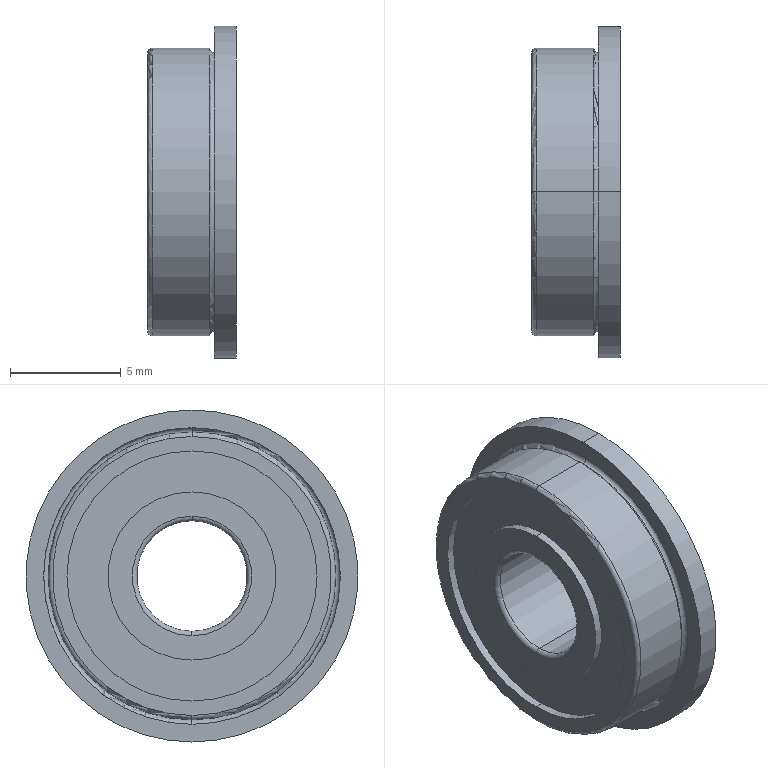Part | SolidWorks | features RefAxis 3, 3DProfileFeature 1, Revolution 1 | 1 solid | 31 faces | box 4 x 15 x 15 mm | volume 450.56 mm3 | cylinder 14 | torus 10 | plane 7 | commonest cylinder face diameters 7.6 x4 11.3 x4 5 x2 13 x2 15 x2
STEP:
#1=CARTESIAN_POINT('',(2.8,0.,6.5));
#2=VERTEX_POINT('',#1);
#3=CARTESIAN_POINT('',(3.,0.,6.3));
#4=VERTEX_POINT('',#3);
#5=CARTESIAN_POINT('',(3.,0.,6.5));
#6=DIRECTION('',(0.,-1.,0.));
#7=DIRECTION('',(0.,0.,-1.));
#8=AXIS2_PLACEMENT_3D('',#5,#6,#7);
#9=CIRCLE('',#8,0.2);
#10=EDGE_CURVE('',#2,#4,#9,.T.);
#11=ORIENTED_EDGE('',*,*,#10,.T.);
#12=CARTESIAN_POINT('',(3.,0.,-6.3));
#13=VERTEX_POINT('',#12);
#14=CARTESIAN_POINT('',(3.,0.,0.));
#15=DIRECTION('',(-1.,0.,0.));
#16=DIRECTION('',(0.,0.,1.));
#17=AXIS2_PLACEMENT_3D('',#14,#15,#16);
#18=CIRCLE('',#17,6.3);
#19=EDGE_CURVE('',#4,#13,#18,.T.);
#20=ORIENTED_EDGE('',*,*,#19,.T.);
#21=CARTESIAN_POINT('',(2.8,0.,-6.5));
#22=VERTEX_POINT('',#21);
#23=CARTESIAN_POINT('',(3.,0.,-6.5));
#24=DIRECTION('',(0.,1.,0.));
#25=DIRECTION('',(0.,0.,1.));
#26=AXIS2_PLACEMENT_3D('',#23,#24,#25);
#27=CIRCLE('',#26,0.2);
#28=EDGE_CURVE('',#22,#13,#27,.T.);
#29=ORIENTED_EDGE('',*,*,#28,.F.);
#30=CARTESIAN_POINT('',(2.8,0.,0.));
#31=DIRECTION('',(-1.,0.,0.));
#32=DIRECTION('',(0.,0.,1.));
#33=AXIS2_PLACEMENT_3D('',#30,#31,#32);
#34=CIRCLE('',#33,6.5);
#35=EDGE_CURVE('',#2,#22,#34,.T.);
#36=ORIENTED_EDGE('',*,*,#35,.F.);
#37=EDGE_LOOP('',(#11,#20,#29,#36));
#38=FACE_OUTER_BOUND('',#37,.T.);
#39=CARTESIAN_POINT('',(3.,0.,0.));
#40=DIRECTION('',(-1.,0.,0.));
#41=DIRECTION('',(0.,0.,1.));
#42=AXIS2_PLACEMENT_3D('',#39,#40,#41);
#43=TOROIDAL_SURFACE('',#42,6.5,0.2);
#44=ADVANCED_FACE('',(#38),#43,.F.);
#45=ORIENTED_EDGE('',*,*,#28,.T.);
#46=CARTESIAN_POINT('',(3.,0.,0.));
#47=DIRECTION('',(-1.,0.,0.));
#48=DIRECTION('',(0.,0.,1.));
#49=AXIS2_PLACEMENT_3D('',#46,#47,#48);
#50=CIRCLE('',#49,6.3);
#51=EDGE_CURVE('',#13,#4,#50,.T.);
#52=ORIENTED_EDGE('',*,*,#51,.T.);
#53=ORIENTED_EDGE('',*,*,#10,.F.);
#54=CARTESIAN_POINT('',(2.8,0.,0.));
#55=DIRECTION('',(-1.,0.,0.));
#56=DIRECTION('',(0.,0.,1.));
#57=AXIS2_PLACEMENT_3D('',#54,#55,#56);
#58=CIRCLE('',#57,6.5);
#59=EDGE_CURVE('',#22,#2,#58,.T.);
#60=ORIENTED_EDGE('',*,*,#59,.F.);
#61=EDGE_LOOP('',(#45,#52,#53,#60));
#62=FACE_OUTER_BOUND('',#61,.T.);
#63=CARTESIAN_POINT('',(3.,0.,0.));
#64=DIRECTION('',(-1.,0.,0.));
#65=DIRECTION('',(0.,0.,1.));
#66=AXIS2_PLACEMENT_3D('',#63,#64,#65);
#67=TOROIDAL_SURFACE('',#66,6.5,0.2);
#68=ADVANCED_FACE('',(#62),#67,.F.);
#69=ORIENTED_EDGE('',*,*,#35,.T.);
#70=CARTESIAN_POINT('',(0.2,0.,-6.5));
#71=VERTEX_POINT('',#70);
#72=CARTESIAN_POINT('',(13.,0.,-6.5));
#73=DIRECTION('',(-1.,0.,0.));
#74=VECTOR('',#73,1000.);
#75=LINE('',#72,#74);
#76=EDGE_CURVE('',#22,#71,#75,.T.);
#77=ORIENTED_EDGE('',*,*,#76,.T.);
#78=CARTESIAN_POINT('',(0.2,0.,6.5));
#79=VERTEX_POINT('',#78);
#80=CARTESIAN_POINT('',(0.2,0.,0.));
#81=DIRECTION('',(-1.,0.,0.));
#82=DIRECTION('',(0.,0.,1.));
#83=AXIS2_PLACEMENT_3D('',#80,#81,#82);
#84=CIRCLE('',#83,6.5);
#85=EDGE_CURVE('',#79,#71,#84,.T.);
#86=ORIENTED_EDGE('',*,*,#85,.F.);
#87=CARTESIAN_POINT('',(13.,0.,6.5));
#88=DIRECTION('',(-1.,0.,0.));
#89=VECTOR('',#88,1000.);
#90=LINE('',#87,#89);
#91=EDGE_CURVE('',#2,#79,#90,.T.);
#92=ORIENTED_EDGE('',*,*,#91,.F.);
#93=EDGE_LOOP('',(#69,#77,#86,#92));
#94=FACE_OUTER_BOUND('',#93,.T.);
#95=CARTESIAN_POINT('',(13.,0.,0.));
#96=DIRECTION('',(-1.,0.,0.));
#97=DIRECTION('',(0.,0.,1.));
#98=AXIS2_PLACEMENT_3D('',#95,#96,#97);
#99=CYLINDRICAL_SURFACE('',#98,6.5);
#100=ADVANCED_FACE('',(#94),#99,.T.);
#101=ORIENTED_EDGE('',*,*,#51,.F.);
#102=CARTESIAN_POINT('',(3.,0.,-6.7));
#103=VERTEX_POINT('',#102);
#104=CARTESIAN_POINT('',(3.,0.,-6.5));
#105=DIRECTION('',(0.,1.,0.));
#106=DIRECTION('',(0.,0.,1.));
#107=AXIS2_PLACEMENT_3D('',#104,#105,#106);
#108=CIRCLE('',#107,0.2);
#109=EDGE_CURVE('',#13,#103,#108,.T.);
#110=ORIENTED_EDGE('',*,*,#109,.T.);
#111=CARTESIAN_POINT('',(3.,0.,6.7));
#112=VERTEX_POINT('',#111);
#113=CARTESIAN_POINT('',(3.,0.,0.));
#114=DIRECTION('',(-1.,0.,0.));
#115=DIRECTION('',(0.,0.,1.));
#116=AXIS2_PLACEMENT_3D('',#113,#114,#115);
#117=CIRCLE('',#116,6.7);
#118=EDGE_CURVE('',#103,#112,#117,.T.);
#119=ORIENTED_EDGE('',*,*,#118,.T.);
#120=CARTESIAN_POINT('',(3.,0.,6.5));
#121=DIRECTION('',(0.,-1.,0.));
#122=DIRECTION('',(0.,0.,-1.));
#123=AXIS2_PLACEMENT_3D('',#120,#121,#122);
#124=CIRCLE('',#123,0.2);
#125=EDGE_CURVE('',#4,#112,#124,.T.);
#126=ORIENTED_EDGE('',*,*,#125,.F.);
#127=EDGE_LOOP('',(#101,#110,#119,#126));
#128=FACE_OUTER_BOUND('',#127,.T.);
#129=CARTESIAN_POINT('',(3.,0.,0.));
#130=DIRECTION('',(-1.,0.,0.));
#131=DIRECTION('',(0.,0.,1.));
#132=AXIS2_PLACEMENT_3D('',#129,#130,#131);
#133=TOROIDAL_SURFACE('',#132,6.5,0.2);
#134=ADVANCED_FACE('',(#128),#133,.F.);
#135=CARTESIAN_POINT('',(4.,0.,7.5));
#136=VERTEX_POINT('',#135);
#137=CARTESIAN_POINT('',(4.,0.,-7.5));
#138=VERTEX_POINT('',#137);
#139=CARTESIAN_POINT('',(4.,0.,0.));
#140=DIRECTION('',(-1.,0.,0.));
#141=DIRECTION('',(0.,0.,1.));
#142=AXIS2_PLACEMENT_3D('',#139,#140,#141);
#143=CIRCLE('',#142,7.5);
#144=EDGE_CURVE('',#136,#138,#143,.T.);
#145=ORIENTED_EDGE('',*,*,#144,.T.);
#146=CARTESIAN_POINT('',(3.,0.,-7.5));
#147=VERTEX_POINT('',#146);
#148=CARTESIAN_POINT('',(13.,0.,-7.5));
#149=DIRECTION('',(-1.,0.,0.));
#150=VECTOR('',#149,1000.);
#151=LINE('',#148,#150);
#152=EDGE_CURVE('',#138,#147,#151,.T.);
#153=ORIENTED_EDGE('',*,*,#152,.T.);
#154=CARTESIAN_POINT('',(3.,0.,7.5));
#155=VERTEX_POINT('',#154);
#156=CARTESIAN_POINT('',(3.,0.,0.));
#157=DIRECTION('',(-1.,0.,0.));
#158=DIRECTION('',(0.,0.,1.));
#159=AXIS2_PLACEMENT_3D('',#156,#157,#158);
#160=CIRCLE('',#159,7.5);
#161=EDGE_CURVE('',#155,#147,#160,.T.);
#162=ORIENTED_EDGE('',*,*,#161,.F.);
#163=CARTESIAN_POINT('',(13.,0.,7.5));
#164=DIRECTION('',(-1.,0.,0.));
#165=VECTOR('',#164,1000.);
#166=LINE('',#163,#165);
#167=EDGE_CURVE('',#136,#155,#166,.T.);
#168=ORIENTED_EDGE('',*,*,#167,.F.);
#169=EDGE_LOOP('',(#145,#153,#162,#168));
#170=FACE_OUTER_BOUND('',#169,.T.);
#171=CARTESIAN_POINT('',(13.,0.,0.));
#172=DIRECTION('',(-1.,0.,0.));
#173=DIRECTION('',(0.,0.,1.));
#174=AXIS2_PLACEMENT_3D('',#171,#172,#173);
#175=CYLINDRICAL_SURFACE('',#174,7.5);
#176=ADVANCED_FACE('',(#170),#175,.T.);
#177=CARTESIAN_POINT('',(4.,0.,-5.65));
#178=VERTEX_POINT('',#177);
#179=CARTESIAN_POINT('',(4.,0.,5.65));
#180=VERTEX_POINT('',#179);
#181=CARTESIAN_POINT('',(4.,0.,0.));
#182=DIRECTION('',(-1.,0.,0.));
#183=DIRECTION('',(0.,0.,1.));
#184=AXIS2_PLACEMENT_3D('',#181,#182,#183);
#185=CIRCLE('',#184,5.65);
#186=EDGE_CURVE('',#178,#180,#185,.T.);
#187=ORIENTED_EDGE('',*,*,#186,.F.);
#188=CARTESIAN_POINT('',(3.623,0.,-5.65));
#189=VERTEX_POINT('',#188);
#190=CARTESIAN_POINT('',(13.,0.,-5.65));
#191=DIRECTION('',(-1.,0.,0.));
#192=VECTOR('',#191,1000.);
#193=LINE('',#190,#192);
#194=EDGE_CURVE('',#178,#189,#193,.T.);
#195=ORIENTED_EDGE('',*,*,#194,.T.);
#196=CARTESIAN_POINT('',(3.623,0.,5.65));
#197=VERTEX_POINT('',#196);
#198=CARTESIAN_POINT('',(3.623,0.,0.));
#199=DIRECTION('',(-1.,0.,0.));
#200=DIRECTION('',(0.,0.,1.));
#201=AXIS2_PLACEMENT_3D('',#198,#199,#200);
#202=CIRCLE('',#201,5.65);
#203=EDGE_CURVE('',#189,#197,#202,.T.);
#204=ORIENTED_EDGE('',*,*,#203,.T.);
#205=CARTESIAN_POINT('',(13.,0.,5.65));
#206=DIRECTION('',(-1.,0.,0.));
#207=VECTOR('',#206,1000.);
#208=LINE('',#205,#207);
#209=EDGE_CURVE('',#180,#197,#208,.T.);
#210=ORIENTED_EDGE('',*,*,#209,.F.);
#211=EDGE_LOOP('',(#187,#195,#204,#210));
#212=FACE_OUTER_BOUND('',#211,.T.);
#213=CARTESIAN_POINT('',(13.,0.,0.));
#214=DIRECTION('',(-1.,0.,0.));
#215=DIRECTION('',(0.,0.,1.));
#216=AXIS2_PLACEMENT_3D('',#213,#214,#215);
#217=CYLINDRICAL_SURFACE('',#216,5.65);
#218=ADVANCED_FACE('',(#212),#217,.F.);
#219=CARTESIAN_POINT('',(4.,0.,3.8));
#220=VERTEX_POINT('',#219);
#221=CARTESIAN_POINT('',(4.,0.,-3.8));
#222=VERTEX_POINT('',#221);
#223=CARTESIAN_POINT('',(4.,0.,0.));
#224=DIRECTION('',(-1.,0.,0.));
#225=DIRECTION('',(0.,0.,1.));
#226=AXIS2_PLACEMENT_3D('',#223,#224,#225);
#227=CIRCLE('',#226,3.8);
#228=EDGE_CURVE('',#220,#222,#227,.T.);
#229=ORIENTED_EDGE('',*,*,#228,.T.);
#230=CARTESIAN_POINT('',(3.623,0.,-3.8));
#231=VERTEX_POINT('',#230);
#232=CARTESIAN_POINT('',(13.,0.,-3.8));
#233=DIRECTION('',(-1.,0.,0.));
#234=VECTOR('',#233,1000.);
#235=LINE('',#232,#234);
#236=EDGE_CURVE('',#222,#231,#235,.T.);
#237=ORIENTED_EDGE('',*,*,#236,.T.);
#238=CARTESIAN_POINT('',(3.623,0.,3.8));
#239=VERTEX_POINT('',#238);
#240=CARTESIAN_POINT('',(3.623,0.,0.));
#241=DIRECTION('',(-1.,0.,0.));
#242=DIRECTION('',(0.,0.,1.));
#243=AXIS2_PLACEMENT_3D('',#240,#241,#242);
#244=CIRCLE('',#243,3.8);
#245=EDGE_CURVE('',#239,#231,#244,.T.);
#246=ORIENTED_EDGE('',*,*,#245,.F.);
#247=CARTESIAN_POINT('',(13.,0.,3.8));
#248=DIRECTION('',(-1.,0.,0.));
#249=VECTOR('',#248,1000.);
#250=LINE('',#247,#249);
#251=EDGE_CURVE('',#220,#239,#250,.T.);
#252=ORIENTED_EDGE('',*,*,#251,.F.);
#253=EDGE_LOOP('',(#229,#237,#246,#252));
#254=FACE_OUTER_BOUND('',#253,.T.);
#255=CARTESIAN_POINT('',(13.,0.,0.));
#256=DIRECTION('',(-1.,0.,0.));
#257=DIRECTION('',(0.,0.,1.));
#258=AXIS2_PLACEMENT_3D('',#255,#256,#257);
#259=CYLINDRICAL_SURFACE('',#258,3.8);
#260=ADVANCED_FACE('',(#254),#259,.T.);
#261=CARTESIAN_POINT('',(3.8,0.,2.5));
#262=VERTEX_POINT('',#261);
#263=CARTESIAN_POINT('',(3.8,0.,-2.5));
#264=VERTEX_POINT('',#263);
#265=CARTESIAN_POINT('',(3.8,0.,0.));
#266=DIRECTION('',(-1.,0.,0.));
#267=DIRECTION('',(0.,0.,1.));
#268=AXIS2_PLACEMENT_3D('',#265,#266,#267);
#269=CIRCLE('',#268,2.5);
#270=EDGE_CURVE('',#262,#264,#269,.T.);
#271=ORIENTED_EDGE('',*,*,#270,.T.);
#272=CARTESIAN_POINT('',(4.,0.,-2.7));
#273=VERTEX_POINT('',#272);
#274=CARTESIAN_POINT('',(3.8,0.,-2.7));
#275=DIRECTION('',(0.,1.,0.));
#276=DIRECTION('',(0.,0.,1.));
#277=AXIS2_PLACEMENT_3D('',#274,#275,#276);
#278=CIRCLE('',#277,0.2);
#279=EDGE_CURVE('',#264,#273,#278,.T.);
#280=ORIENTED_EDGE('',*,*,#279,.T.);
#281=CARTESIAN_POINT('',(4.,0.,2.7));
#282=VERTEX_POINT('',#281);
#283=CARTESIAN_POINT('',(4.,0.,0.));
#284=DIRECTION('',(-1.,0.,0.));
#285=DIRECTION('',(0.,0.,1.));
#286=AXIS2_PLACEMENT_3D('',#283,#284,#285);
#287=CIRCLE('',#286,2.7);
#288=EDGE_CURVE('',#282,#273,#287,.T.);
#289=ORIENTED_EDGE('',*,*,#288,.F.);
#290=CARTESIAN_POINT('',(3.8,0.,2.7));
#291=DIRECTION('',(0.,-1.,0.));
#292=DIRECTION('',(0.,0.,-1.));
#293=AXIS2_PLACEMENT_3D('',#290,#291,#292);
#294=CIRCLE('',#293,0.2);
#295=EDGE_CURVE('',#262,#282,#294,.T.);
#296=ORIENTED_EDGE('',*,*,#295,.F.);
#297=EDGE_LOOP('',(#271,#280,#289,#296));
#298=FACE_OUTER_BOUND('',#297,.T.);
#299=CARTESIAN_POINT('',(3.8,0.,0.));
#300=DIRECTION('',(-1.,0.,0.));
#301=DIRECTION('',(0.,0.,1.));
#302=AXIS2_PLACEMENT_3D('',#299,#300,#301);
#303=TOROIDAL_SURFACE('',#302,2.7,0.2);
#304=ADVANCED_FACE('',(#298),#303,.T.);
#305=CARTESIAN_POINT('',(3.8,0.,0.));
#306=DIRECTION('',(-1.,0.,0.));
#307=DIRECTION('',(0.,0.,1.));
#308=AXIS2_PLACEMENT_3D('',#305,#306,#307);
#309=CIRCLE('',#308,2.5);
#310=EDGE_CURVE('',#264,#262,#309,.T.);
#311=ORIENTED_EDGE('',*,*,#310,.F.);
#312=CARTESIAN_POINT('',(0.2,0.,-2.5));
#313=VERTEX_POINT('',#312);
#314=CARTESIAN_POINT('',(13.,0.,-2.5));
#315=DIRECTION('',(-1.,0.,0.));
#316=VECTOR('',#315,1000.);
#317=LINE('',#314,#316);
#318=EDGE_CURVE('',#264,#313,#317,.T.);
#319=ORIENTED_EDGE('',*,*,#318,.T.);
#320=CARTESIAN_POINT('',(0.2,0.,2.5));
#321=VERTEX_POINT('',#320);
#322=CARTESIAN_POINT('',(0.2,0.,0.));
#323=DIRECTION('',(-1.,0.,0.));
#324=DIRECTION('',(0.,0.,1.));
#325=AXIS2_PLACEMENT_3D('',#322,#323,#324);
#326=CIRCLE('',#325,2.5);
#327=EDGE_CURVE('',#313,#321,#326,.T.);
#328=ORIENTED_EDGE('',*,*,#327,.T.);
#329=CARTESIAN_POINT('',(13.,0.,2.5));
#330=DIRECTION('',(-1.,0.,0.));
#331=VECTOR('',#330,1000.);
#332=LINE('',#329,#331);
#333=EDGE_CURVE('',#262,#321,#332,.T.);
#334=ORIENTED_EDGE('',*,*,#333,.F.);
#335=EDGE_LOOP('',(#311,#319,#328,#334));
#336=FACE_OUTER_BOUND('',#335,.T.);
#337=CARTESIAN_POINT('',(13.,0.,0.));
#338=DIRECTION('',(-1.,0.,0.));
#339=DIRECTION('',(0.,0.,1.));
#340=AXIS2_PLACEMENT_3D('',#337,#338,#339);
#341=CYLINDRICAL_SURFACE('',#340,2.5);
#342=ADVANCED_FACE('',(#336),#341,.F.);
#343=CARTESIAN_POINT('',(0.,0.,2.7));
#344=VERTEX_POINT('',#343);
#345=CARTESIAN_POINT('',(0.,0.,-2.7));
#346=VERTEX_POINT('',#345);
#347=CARTESIAN_POINT('',(0.,0.,0.));
#348=DIRECTION('',(-1.,0.,0.));
#349=DIRECTION('',(0.,0.,1.));
#350=AXIS2_PLACEMENT_3D('',#347,#348,#349);
#351=CIRCLE('',#350,2.7);
#352=EDGE_CURVE('',#344,#346,#351,.T.);
#353=ORIENTED_EDGE('',*,*,#352,.T.);
#354=CARTESIAN_POINT('',(0.2,0.,-2.7));
#355=DIRECTION('',(0.,1.,0.));
#356=DIRECTION('',(0.,0.,1.));
#357=AXIS2_PLACEMENT_3D('',#354,#355,#356);
#358=CIRCLE('',#357,0.2);
#359=EDGE_CURVE('',#346,#313,#358,.T.);
#360=ORIENTED_EDGE('',*,*,#359,.T.);
#361=CARTESIAN_POINT('',(0.2,0.,0.));
#362=DIRECTION('',(-1.,0.,0.));
#363=DIRECTION('',(0.,0.,1.));
#364=AXIS2_PLACEMENT_3D('',#361,#362,#363);
#365=CIRCLE('',#364,2.5);
#366=EDGE_CURVE('',#321,#313,#365,.T.);
#367=ORIENTED_EDGE('',*,*,#366,.F.);
#368=CARTESIAN_POINT('',(0.2,0.,2.7));
#369=DIRECTION('',(0.,-1.,0.));
#370=DIRECTION('',(0.,0.,-1.));
#371=AXIS2_PLACEMENT_3D('',#368,#369,#370);
#372=CIRCLE('',#371,0.2);
#373=EDGE_CURVE('',#344,#321,#372,.T.);
#374=ORIENTED_EDGE('',*,*,#373,.F.);
#375=EDGE_LOOP('',(#353,#360,#367,#374));
#376=FACE_OUTER_BOUND('',#375,.T.);
#377=CARTESIAN_POINT('',(0.2,0.,0.));
#378=DIRECTION('',(-1.,0.,0.));
#379=DIRECTION('',(0.,0.,1.));
#380=AXIS2_PLACEMENT_3D('',#377,#378,#379);
#381=TOROIDAL_SURFACE('',#380,2.7,0.2);
#382=ADVANCED_FACE('',(#376),#381,.T.);
#383=CARTESIAN_POINT('',(0.3765,0.,3.8));
#384=VERTEX_POINT('',#383);
#385=CARTESIAN_POINT('',(0.3765,0.,-3.8));
#386=VERTEX_POINT('',#385);
#387=CARTESIAN_POINT('',(0.3765,0.,0.));
#388=DIRECTION('',(-1.,0.,0.));
#389=DIRECTION('',(0.,0.,1.));
#390=AXIS2_PLACEMENT_3D('',#387,#388,#389);
#391=CIRCLE('',#390,3.8);
#392=EDGE_CURVE('',#384,#386,#391,.T.);
#393=ORIENTED_EDGE('',*,*,#392,.T.);
#394=CARTESIAN_POINT('',(0.,0.,-3.8));
#395=VERTEX_POINT('',#394);
#396=CARTESIAN_POINT('',(13.,0.,-3.8));
#397=DIRECTION('',(-1.,0.,0.));
#398=VECTOR('',#397,1000.);
#399=LINE('',#396,#398);
#400=EDGE_CURVE('',#386,#395,#399,.T.);
#401=ORIENTED_EDGE('',*,*,#400,.T.);
#402=CARTESIAN_POINT('',(0.,0.,3.8));
#403=VERTEX_POINT('',#402);
#404=CARTESIAN_POINT('',(0.,0.,0.));
#405=DIRECTION('',(-1.,0.,0.));
#406=DIRECTION('',(0.,0.,1.));
#407=AXIS2_PLACEMENT_3D('',#404,#405,#406);
#408=CIRCLE('',#407,3.8);
#409=EDGE_CURVE('',#403,#395,#408,.T.);
#410=ORIENTED_EDGE('',*,*,#409,.F.);
#411=CARTESIAN_POINT('',(13.,0.,3.8));
#412=DIRECTION('',(-1.,0.,0.));
#413=VECTOR('',#412,1000.);
#414=LINE('',#411,#413);
#415=EDGE_CURVE('',#384,#403,#414,.T.);
#416=ORIENTED_EDGE('',*,*,#415,.F.);
#417=EDGE_LOOP('',(#393,#401,#410,#416));
#418=FACE_OUTER_BOUND('',#417,.T.);
#419=CARTESIAN_POINT('',(13.,0.,0.));
#420=DIRECTION('',(-1.,0.,0.));
#421=DIRECTION('',(0.,0.,1.));
#422=AXIS2_PLACEMENT_3D('',#419,#420,#421);
#423=CYLINDRICAL_SURFACE('',#422,3.8);
#424=ADVANCED_FACE('',(#418),#423,.T.);
#425=CARTESIAN_POINT('',(0.3765,0.,-5.65));
#426=VERTEX_POINT('',#425);
#427=CARTESIAN_POINT('',(0.3765,0.,5.65));
#428=VERTEX_POINT('',#427);
#429=CARTESIAN_POINT('',(0.3765,0.,0.));
#430=DIRECTION('',(-1.,0.,0.));
#431=DIRECTION('',(0.,0.,1.));
#432=AXIS2_PLACEMENT_3D('',#429,#430,#431);
#433=CIRCLE('',#432,5.65);
#434=EDGE_CURVE('',#426,#428,#433,.T.);
#435=ORIENTED_EDGE('',*,*,#434,.F.);
#436=CARTESIAN_POINT('',(0.,0.,-5.65));
#437=VERTEX_POINT('',#436);
#438=CARTESIAN_POINT('',(13.,0.,-5.65));
#439=DIRECTION('',(-1.,0.,0.));
#440=VECTOR('',#439,1000.);
#441=LINE('',#438,#440);
#442=EDGE_CURVE('',#426,#437,#441,.T.);
#443=ORIENTED_EDGE('',*,*,#442,.T.);
#444=CARTESIAN_POINT('',(0.,0.,5.65));
#445=VERTEX_POINT('',#444);
#446=CARTESIAN_POINT('',(0.,0.,0.));
#447=DIRECTION('',(-1.,0.,0.));
#448=DIRECTION('',(0.,0.,1.));
#449=AXIS2_PLACEMENT_3D('',#446,#447,#448);
#450=CIRCLE('',#449,5.65);
#451=EDGE_CURVE('',#437,#445,#450,.T.);
#452=ORIENTED_EDGE('',*,*,#451,.T.);
#453=CARTESIAN_POINT('',(13.,0.,5.65));
#454=DIRECTION('',(-1.,0.,0.));
#455=VECTOR('',#454,1000.);
#456=LINE('',#453,#455);
#457=EDGE_CURVE('',#428,#445,#456,.T.);
#458=ORIENTED_EDGE('',*,*,#457,.F.);
#459=EDGE_LOOP('',(#435,#443,#452,#458));
#460=FACE_OUTER_BOUND('',#459,.T.);
#461=CARTESIAN_POINT('',(13.,0.,0.));
#462=DIRECTION('',(-1.,0.,0.));
#463=DIRECTION('',(0.,0.,1.));
#464=AXIS2_PLACEMENT_3D('',#461,#462,#463);
#465=CYLINDRICAL_SURFACE('',#464,5.65);
#466=ADVANCED_FACE('',(#460),#465,.F.);
#467=ORIENTED_EDGE('',*,*,#85,.T.);
#468=CARTESIAN_POINT('',(0.,0.,-6.3));
#469=VERTEX_POINT('',#468);
#470=CARTESIAN_POINT('',(0.2,0.,-6.3));
#471=DIRECTION('',(0.,1.,0.));
#472=DIRECTION('',(0.,0.,1.));
#473=AXIS2_PLACEMENT_3D('',#470,#471,#472);
#474=CIRCLE('',#473,0.2);
#475=EDGE_CURVE('',#71,#469,#474,.T.);
#476=ORIENTED_EDGE('',*,*,#475,.T.);
#477=CARTESIAN_POINT('',(0.,0.,6.3));
#478=VERTEX_POINT('',#477);
#479=CARTESIAN_POINT('',(0.,0.,0.));
#480=DIRECTION('',(-1.,0.,0.));
#481=DIRECTION('',(0.,0.,1.));
#482=AXIS2_PLACEMENT_3D('',#479,#480,#481);
#483=CIRCLE('',#482,6.3);
#484=EDGE_CURVE('',#478,#469,#483,.T.);
#485=ORIENTED_EDGE('',*,*,#484,.F.);
#486=CARTESIAN_POINT('',(0.2,0.,6.3));
#487=DIRECTION('',(0.,-1.,0.));
#488=DIRECTION('',(0.,0.,-1.));
#489=AXIS2_PLACEMENT_3D('',#486,#487,#488);
#490=CIRCLE('',#489,0.2);
#491=EDGE_CURVE('',#79,#478,#490,.T.);
#492=ORIENTED_EDGE('',*,*,#491,.F.);
#493=EDGE_LOOP('',(#467,#476,#485,#492));
#494=FACE_OUTER_BOUND('',#493,.T.);
#495=CARTESIAN_POINT('',(0.2,0.,0.));
#496=DIRECTION('',(-1.,0.,0.));
#497=DIRECTION('',(0.,0.,1.));
#498=AXIS2_PLACEMENT_3D('',#495,#496,#497);
#499=TOROIDAL_SURFACE('',#498,6.3,0.2);
#500=ADVANCED_FACE('',(#494),#499,.T.);
#501=ORIENTED_EDGE('',*,*,#475,.F.);
#502=CARTESIAN_POINT('',(0.2,0.,0.));
#503=DIRECTION('',(-1.,0.,0.));
#504=DIRECTION('',(0.,0.,1.));
#505=AXIS2_PLACEMENT_3D('',#502,#503,#504);
#506=CIRCLE('',#505,6.5);
#507=EDGE_CURVE('',#71,#79,#506,.T.);
#508=ORIENTED_EDGE('',*,*,#507,.T.);
#509=ORIENTED_EDGE('',*,*,#491,.T.);
#510=CARTESIAN_POINT('',(0.,0.,0.));
#511=DIRECTION('',(-1.,0.,0.));
#512=DIRECTION('',(0.,0.,1.));
#513=AXIS2_PLACEMENT_3D('',#510,#511,#512);
#514=CIRCLE('',#513,6.3);
#515=EDGE_CURVE('',#469,#478,#514,.T.);
#516=ORIENTED_EDGE('',*,*,#515,.F.);
#517=EDGE_LOOP('',(#501,#508,#509,#516));
#518=FACE_OUTER_BOUND('',#517,.T.);
#519=CARTESIAN_POINT('',(0.2,0.,0.));
#520=DIRECTION('',(-1.,0.,0.));
#521=DIRECTION('',(0.,0.,1.));
#522=AXIS2_PLACEMENT_3D('',#519,#520,#521);
#523=TOROIDAL_SURFACE('',#522,6.3,0.2);
#524=ADVANCED_FACE('',(#518),#523,.T.);
#525=CARTESIAN_POINT('',(0.,0.,0.));
#526=DIRECTION('',(-1.,0.,0.));
#527=DIRECTION('',(0.,0.,1.));
#528=AXIS2_PLACEMENT_3D('',#525,#526,#527);
#529=CIRCLE('',#528,5.65);
#530=EDGE_CURVE('',#445,#437,#529,.T.);
#531=ORIENTED_EDGE('',*,*,#530,.F.);
#532=ORIENTED_EDGE('',*,*,#451,.F.);
#533=EDGE_LOOP('',(#531,#532));
#534=FACE_BOUND('',#533,.T.);
#535=ORIENTED_EDGE('',*,*,#484,.T.);
#536=ORIENTED_EDGE('',*,*,#515,.T.);
#537=EDGE_LOOP('',(#535,#536));
#538=FACE_OUTER_BOUND('',#537,.T.);
#539=CARTESIAN_POINT('',(0.,6.3,0.));
#540=DIRECTION('',(1.,0.,0.));
#541=DIRECTION('',(0.,0.,-1.));
#542=AXIS2_PLACEMENT_3D('',#539,#540,#541);
#543=PLANE('',#542);
#544=ADVANCED_FACE('',(#534,#538),#543,.F.);
#545=ORIENTED_EDGE('',*,*,#442,.F.);
#546=CARTESIAN_POINT('',(0.3765,0.,0.));
#547=DIRECTION('',(-1.,0.,0.));
#548=DIRECTION('',(0.,0.,1.));
#549=AXIS2_PLACEMENT_3D('',#546,#547,#548);
#550=CIRCLE('',#549,5.65);
#551=EDGE_CURVE('',#428,#426,#550,.T.);
#552=ORIENTED_EDGE('',*,*,#551,.F.);
#553=ORIENTED_EDGE('',*,*,#457,.T.);
#554=ORIENTED_EDGE('',*,*,#530,.T.);
#555=EDGE_LOOP('',(#545,#552,#553,#554));
#556=FACE_OUTER_BOUND('',#555,.T.);
#557=CARTESIAN_POINT('',(13.,0.,0.));
#558=DIRECTION('',(-1.,0.,0.));
#559=DIRECTION('',(0.,0.,1.));
#560=AXIS2_PLACEMENT_3D('',#557,#558,#559);
#561=CYLINDRICAL_SURFACE('',#560,5.65);
#562=ADVANCED_FACE('',(#556),#561,.F.);
#563=ORIENTED_EDGE('',*,*,#392,.F.);
#564=CARTESIAN_POINT('',(0.3765,0.,0.));
#565=DIRECTION('',(-1.,0.,0.));
#566=DIRECTION('',(0.,0.,1.));
#567=AXIS2_PLACEMENT_3D('',#564,#565,#566);
#568=CIRCLE('',#567,3.8);
#569=EDGE_CURVE('',#386,#384,#568,.T.);
#570=ORIENTED_EDGE('',*,*,#569,.F.);
#571=EDGE_LOOP('',(#563,#570));
#572=FACE_BOUND('',#571,.T.);
#573=ORIENTED_EDGE('',*,*,#551,.T.);
#574=ORIENTED_EDGE('',*,*,#434,.T.);
#575=EDGE_LOOP('',(#573,#574));
#576=FACE_OUTER_BOUND('',#575,.T.);
#577=CARTESIAN_POINT('',(0.3765,5.65,0.));
#578=DIRECTION('',(1.,0.,0.));
#579=DIRECTION('',(0.,0.,-1.));
#580=AXIS2_PLACEMENT_3D('',#577,#578,#579);
#581=PLANE('',#580);
#582=ADVANCED_FACE('',(#572,#576),#581,.F.);
#583=ORIENTED_EDGE('',*,*,#400,.F.);
#584=ORIENTED_EDGE('',*,*,#569,.T.);
#585=ORIENTED_EDGE('',*,*,#415,.T.);
#586=CARTESIAN_POINT('',(0.,0.,0.));
#587=DIRECTION('',(-1.,0.,0.));
#588=DIRECTION('',(0.,0.,1.));
#589=AXIS2_PLACEMENT_3D('',#586,#587,#588);
#590=CIRCLE('',#589,3.8);
#591=EDGE_CURVE('',#395,#403,#590,.T.);
#592=ORIENTED_EDGE('',*,*,#591,.F.);
#593=EDGE_LOOP('',(#583,#584,#585,#592));
#594=FACE_OUTER_BOUND('',#593,.T.);
#595=CARTESIAN_POINT('',(13.,0.,0.));
#596=DIRECTION('',(-1.,0.,0.));
#597=DIRECTION('',(0.,0.,1.));
#598=AXIS2_PLACEMENT_3D('',#595,#596,#597);
#599=CYLINDRICAL_SURFACE('',#598,3.8);
#600=ADVANCED_FACE('',(#594),#599,.T.);
#601=ORIENTED_EDGE('',*,*,#352,.F.);
#602=CARTESIAN_POINT('',(0.,0.,0.));
#603=DIRECTION('',(-1.,0.,0.));
#604=DIRECTION('',(0.,0.,1.));
#605=AXIS2_PLACEMENT_3D('',#602,#603,#604);
#606=CIRCLE('',#605,2.7);
#607=EDGE_CURVE('',#346,#344,#606,.T.);
#608=ORIENTED_EDGE('',*,*,#607,.F.);
#609=EDGE_LOOP('',(#601,#608));
#610=FACE_BOUND('',#609,.T.);
#611=ORIENTED_EDGE('',*,*,#409,.T.);
#612=ORIENTED_EDGE('',*,*,#591,.T.);
#613=EDGE_LOOP('',(#611,#612));
#614=FACE_OUTER_BOUND('',#613,.T.);
#615=CARTESIAN_POINT('',(0.,3.8,0.));
#616=DIRECTION('',(1.,0.,0.));
#617=DIRECTION('',(0.,0.,-1.));
#618=AXIS2_PLACEMENT_3D('',#615,#616,#617);
#619=PLANE('',#618);
#620=ADVANCED_FACE('',(#610,#614),#619,.F.);
#621=ORIENTED_EDGE('',*,*,#359,.F.);
#622=ORIENTED_EDGE('',*,*,#607,.T.);
#623=ORIENTED_EDGE('',*,*,#373,.T.);
#624=ORIENTED_EDGE('',*,*,#327,.F.);
#625=EDGE_LOOP('',(#621,#622,#623,#624));
#626=FACE_OUTER_BOUND('',#625,.T.);
#627=CARTESIAN_POINT('',(0.2,0.,0.));
#628=DIRECTION('',(-1.,0.,0.));
#629=DIRECTION('',(0.,0.,1.));
#630=AXIS2_PLACEMENT_3D('',#627,#628,#629);
#631=TOROIDAL_SURFACE('',#630,2.7,0.2);
#632=ADVANCED_FACE('',(#626),#631,.T.);
#633=ORIENTED_EDGE('',*,*,#318,.F.);
#634=ORIENTED_EDGE('',*,*,#270,.F.);
#635=ORIENTED_EDGE('',*,*,#333,.T.);
#636=ORIENTED_EDGE('',*,*,#366,.T.);
#637=EDGE_LOOP('',(#633,#634,#635,#636));
#638=FACE_OUTER_BOUND('',#637,.T.);
#639=CARTESIAN_POINT('',(13.,0.,0.));
#640=DIRECTION('',(-1.,0.,0.));
#641=DIRECTION('',(0.,0.,1.));
#642=AXIS2_PLACEMENT_3D('',#639,#640,#641);
#643=CYLINDRICAL_SURFACE('',#642,2.5);
#644=ADVANCED_FACE('',(#638),#643,.F.);
#645=ORIENTED_EDGE('',*,*,#279,.F.);
#646=ORIENTED_EDGE('',*,*,#310,.T.);
#647=ORIENTED_EDGE('',*,*,#295,.T.);
#648=CARTESIAN_POINT('',(4.,0.,0.));
#649=DIRECTION('',(-1.,0.,0.));
#650=DIRECTION('',(0.,0.,1.));
#651=AXIS2_PLACEMENT_3D('',#648,#649,#650);
#652=CIRCLE('',#651,2.7);
#653=EDGE_CURVE('',#273,#282,#652,.T.);
#654=ORIENTED_EDGE('',*,*,#653,.F.);
#655=EDGE_LOOP('',(#645,#646,#647,#654));
#656=FACE_OUTER_BOUND('',#655,.T.);
#657=CARTESIAN_POINT('',(3.8,0.,0.));
#658=DIRECTION('',(-1.,0.,0.));
#659=DIRECTION('',(0.,0.,1.));
#660=AXIS2_PLACEMENT_3D('',#657,#658,#659);
#661=TOROIDAL_SURFACE('',#660,2.7,0.2);
#662=ADVANCED_FACE('',(#656),#661,.T.);
#663=ORIENTED_EDGE('',*,*,#228,.F.);
#664=CARTESIAN_POINT('',(4.,0.,0.));
#665=DIRECTION('',(-1.,0.,0.));
#666=DIRECTION('',(0.,0.,1.));
#667=AXIS2_PLACEMENT_3D('',#664,#665,#666);
#668=CIRCLE('',#667,3.8);
#669=EDGE_CURVE('',#222,#220,#668,.T.);
#670=ORIENTED_EDGE('',*,*,#669,.F.);
#671=EDGE_LOOP('',(#663,#670));
#672=FACE_OUTER_BOUND('',#671,.T.);
#673=ORIENTED_EDGE('',*,*,#288,.T.);
#674=ORIENTED_EDGE('',*,*,#653,.T.);
#675=EDGE_LOOP('',(#673,#674));
#676=FACE_BOUND('',#675,.T.);
#677=CARTESIAN_POINT('',(4.,2.7,0.));
#678=DIRECTION('',(-1.,0.,0.));
#679=DIRECTION('',(0.,0.,1.));
#680=AXIS2_PLACEMENT_3D('',#677,#678,#679);
#681=PLANE('',#680);
#682=ADVANCED_FACE('',(#672,#676),#681,.F.);
#683=ORIENTED_EDGE('',*,*,#236,.F.);
#684=ORIENTED_EDGE('',*,*,#669,.T.);
#685=ORIENTED_EDGE('',*,*,#251,.T.);
#686=CARTESIAN_POINT('',(3.623,0.,0.));
#687=DIRECTION('',(-1.,0.,0.));
#688=DIRECTION('',(0.,0.,1.));
#689=AXIS2_PLACEMENT_3D('',#686,#687,#688);
#690=CIRCLE('',#689,3.8);
#691=EDGE_CURVE('',#231,#239,#690,.T.);
#692=ORIENTED_EDGE('',*,*,#691,.F.);
#693=EDGE_LOOP('',(#683,#684,#685,#692));
#694=FACE_OUTER_BOUND('',#693,.T.);
#695=CARTESIAN_POINT('',(13.,0.,0.));
#696=DIRECTION('',(-1.,0.,0.));
#697=DIRECTION('',(0.,0.,1.));
#698=AXIS2_PLACEMENT_3D('',#695,#696,#697);
#699=CYLINDRICAL_SURFACE('',#698,3.8);
#700=ADVANCED_FACE('',(#694),#699,.T.);
#701=CARTESIAN_POINT('',(3.623,0.,0.));
#702=DIRECTION('',(-1.,0.,0.));
#703=DIRECTION('',(0.,0.,1.));
#704=AXIS2_PLACEMENT_3D('',#701,#702,#703);
#705=CIRCLE('',#704,5.65);
#706=EDGE_CURVE('',#197,#189,#705,.T.);
#707=ORIENTED_EDGE('',*,*,#706,.F.);
#708=ORIENTED_EDGE('',*,*,#203,.F.);
#709=EDGE_LOOP('',(#707,#708));
#710=FACE_OUTER_BOUND('',#709,.T.);
#711=ORIENTED_EDGE('',*,*,#245,.T.);
#712=ORIENTED_EDGE('',*,*,#691,.T.);
#713=EDGE_LOOP('',(#711,#712));
#714=FACE_BOUND('',#713,.T.);
#715=CARTESIAN_POINT('',(3.623,3.8,0.));
#716=DIRECTION('',(-1.,0.,0.));
#717=DIRECTION('',(0.,0.,1.));
#718=AXIS2_PLACEMENT_3D('',#715,#716,#717);
#719=PLANE('',#718);
#720=ADVANCED_FACE('',(#710,#714),#719,.F.);
#721=ORIENTED_EDGE('',*,*,#194,.F.);
#722=CARTESIAN_POINT('',(4.,0.,0.));
#723=DIRECTION('',(-1.,0.,0.));
#724=DIRECTION('',(0.,0.,1.));
#725=AXIS2_PLACEMENT_3D('',#722,#723,#724);
#726=CIRCLE('',#725,5.65);
#727=EDGE_CURVE('',#180,#178,#726,.T.);
#728=ORIENTED_EDGE('',*,*,#727,.F.);
#729=ORIENTED_EDGE('',*,*,#209,.T.);
#730=ORIENTED_EDGE('',*,*,#706,.T.);
#731=EDGE_LOOP('',(#721,#728,#729,#730));
#732=FACE_OUTER_BOUND('',#731,.T.);
#733=CARTESIAN_POINT('',(13.,0.,0.));
#734=DIRECTION('',(-1.,0.,0.));
#735=DIRECTION('',(0.,0.,1.));
#736=AXIS2_PLACEMENT_3D('',#733,#734,#735);
#737=CYLINDRICAL_SURFACE('',#736,5.65);
#738=ADVANCED_FACE('',(#732),#737,.F.);
#739=ORIENTED_EDGE('',*,*,#144,.F.);
#740=CARTESIAN_POINT('',(4.,0.,0.));
#741=DIRECTION('',(-1.,0.,0.));
#742=DIRECTION('',(0.,0.,1.));
#743=AXIS2_PLACEMENT_3D('',#740,#741,#742);
#744=CIRCLE('',#743,7.5);
#745=EDGE_CURVE('',#138,#136,#744,.T.);
#746=ORIENTED_EDGE('',*,*,#745,.F.);
#747=EDGE_LOOP('',(#739,#746));
#748=FACE_OUTER_BOUND('',#747,.T.);
#749=ORIENTED_EDGE('',*,*,#727,.T.);
#750=ORIENTED_EDGE('',*,*,#186,.T.);
#751=EDGE_LOOP('',(#749,#750));
#752=FACE_BOUND('',#751,.T.);
#753=CARTESIAN_POINT('',(4.,5.65,0.));
#754=DIRECTION('',(-1.,0.,0.));
#755=DIRECTION('',(0.,0.,1.));
#756=AXIS2_PLACEMENT_3D('',#753,#754,#755);
#757=PLANE('',#756);
#758=ADVANCED_FACE('',(#748,#752),#757,.F.);
#759=ORIENTED_EDGE('',*,*,#152,.F.);
#760=ORIENTED_EDGE('',*,*,#745,.T.);
#761=ORIENTED_EDGE('',*,*,#167,.T.);
#762=CARTESIAN_POINT('',(3.,0.,0.));
#763=DIRECTION('',(-1.,0.,0.));
#764=DIRECTION('',(0.,0.,1.));
#765=AXIS2_PLACEMENT_3D('',#762,#763,#764);
#766=CIRCLE('',#765,7.5);
#767=EDGE_CURVE('',#147,#155,#766,.T.);
#768=ORIENTED_EDGE('',*,*,#767,.F.);
#769=EDGE_LOOP('',(#759,#760,#761,#768));
#770=FACE_OUTER_BOUND('',#769,.T.);
#771=CARTESIAN_POINT('',(13.,0.,0.));
#772=DIRECTION('',(-1.,0.,0.));
#773=DIRECTION('',(0.,0.,1.));
#774=AXIS2_PLACEMENT_3D('',#771,#772,#773);
#775=CYLINDRICAL_SURFACE('',#774,7.5);
#776=ADVANCED_FACE('',(#770),#775,.T.);
#777=CARTESIAN_POINT('',(3.,0.,0.));
#778=DIRECTION('',(-1.,0.,0.));
#779=DIRECTION('',(0.,0.,1.));
#780=AXIS2_PLACEMENT_3D('',#777,#778,#779);
#781=CIRCLE('',#780,6.7);
#782=EDGE_CURVE('',#112,#103,#781,.T.);
#783=ORIENTED_EDGE('',*,*,#782,.F.);
#784=ORIENTED_EDGE('',*,*,#118,.F.);
#785=EDGE_LOOP('',(#783,#784));
#786=FACE_BOUND('',#785,.T.);
#787=ORIENTED_EDGE('',*,*,#161,.T.);
#788=ORIENTED_EDGE('',*,*,#767,.T.);
#789=EDGE_LOOP('',(#787,#788));
#790=FACE_OUTER_BOUND('',#789,.T.);
#791=CARTESIAN_POINT('',(3.,7.5,0.));
#792=DIRECTION('',(1.,0.,0.));
#793=DIRECTION('',(0.,0.,-1.));
#794=AXIS2_PLACEMENT_3D('',#791,#792,#793);
#795=PLANE('',#794);
#796=ADVANCED_FACE('',(#786,#790),#795,.F.);
#797=ORIENTED_EDGE('',*,*,#19,.F.);
#798=ORIENTED_EDGE('',*,*,#125,.T.);
#799=ORIENTED_EDGE('',*,*,#782,.T.);
#800=ORIENTED_EDGE('',*,*,#109,.F.);
#801=EDGE_LOOP('',(#797,#798,#799,#800));
#802=FACE_OUTER_BOUND('',#801,.T.);
#803=CARTESIAN_POINT('',(3.,0.,0.));
#804=DIRECTION('',(-1.,0.,0.));
#805=DIRECTION('',(0.,0.,1.));
#806=AXIS2_PLACEMENT_3D('',#803,#804,#805);
#807=TOROIDAL_SURFACE('',#806,6.5,0.2);
#808=ADVANCED_FACE('',(#802),#807,.F.);
#809=ORIENTED_EDGE('',*,*,#76,.F.);
#810=ORIENTED_EDGE('',*,*,#59,.T.);
#811=ORIENTED_EDGE('',*,*,#91,.T.);
#812=ORIENTED_EDGE('',*,*,#507,.F.);
#813=EDGE_LOOP('',(#809,#810,#811,#812));
#814=FACE_OUTER_BOUND('',#813,.T.);
#815=CARTESIAN_POINT('',(13.,0.,0.));
#816=DIRECTION('',(-1.,0.,0.));
#817=DIRECTION('',(0.,0.,1.));
#818=AXIS2_PLACEMENT_3D('',#815,#816,#817);
#819=CYLINDRICAL_SURFACE('',#818,6.5);
#820=ADVANCED_FACE('',(#814),#819,.T.);
#821=CLOSED_SHELL('',(#44,#68,#100,#134,#176,#218,#260,#304,#342,#382,#424,#466,#500,#524,#544,#562,#582,#600,#620,#632,#644,#662,#682,#700,#720,#738,#758,#776,#796,#808,#820));
#822=MANIFOLD_SOLID_BREP('',#821);
#823=CARTESIAN_POINT('',(0.,0.,0.));
#824=DIRECTION('',(0.,0.,1.));
#825=DIRECTION('',(1.,0.,0.));
#826=AXIS2_PLACEMENT_3D('',#823,#824,#825);
#827=(LENGTH_UNIT()NAMED_UNIT(*)SI_UNIT(.MILLI.,.METRE.));
#828=UNCERTAINTY_MEASURE_WITH_UNIT(LENGTH_MEASURE(0.00001),#827,'','');
#829=(NAMED_UNIT(*)PLANE_ANGLE_UNIT()SI_UNIT($,.RADIAN.));
#830=(NAMED_UNIT(*)SI_UNIT($,.STERADIAN.)SOLID_ANGLE_UNIT());
#831=(GEOMETRIC_REPRESENTATION_CONTEXT(3)GLOBAL_UNCERTAINTY_ASSIGNED_CONTEXT((#828))GLOBAL_UNIT_ASSIGNED_CONTEXT((#827,#829,#830))REPRESENTATION_CONTEXT('',''));
#832=ADVANCED_BREP_SHAPE_REPRESENTATION('',(#822,#826),#831);